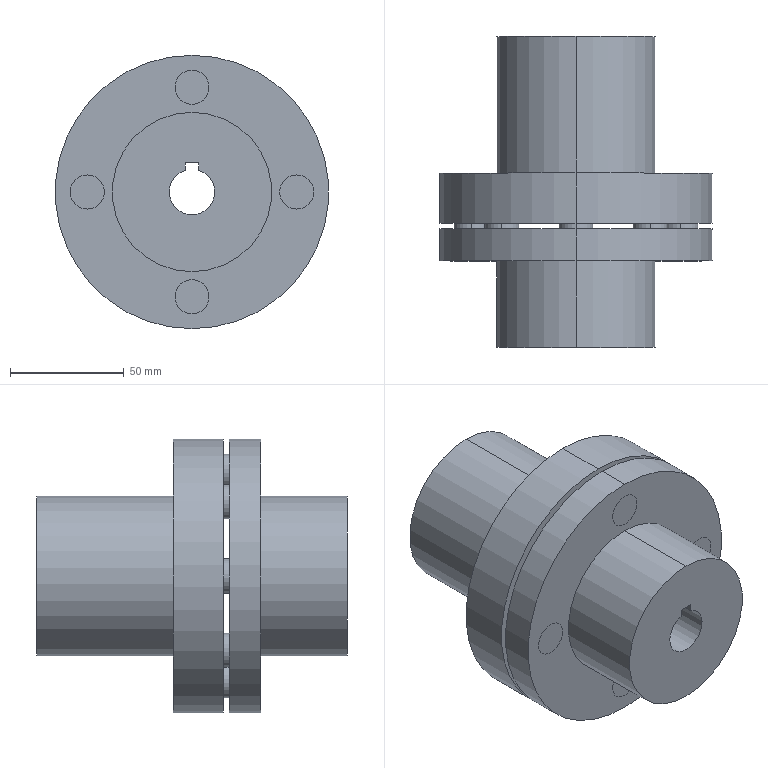Part | SolidWorks | features ICE 6, Revolution 1 | 6 solids | 77 faces | box 120 x 136.5 x 120 mm | volume 665087 mm3 | cylinder 52 | plane 25 | commonest cylinder face diameters 15 x40 70 x4 120 x4 48 x2 20 x1 38 x1